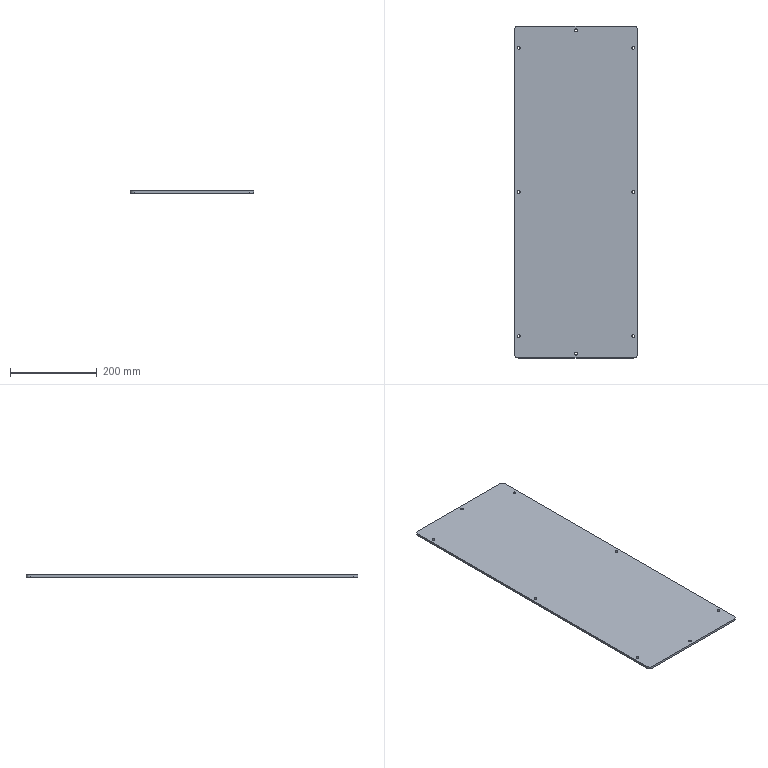Part | STEP file | 1 solid | 26 faces | box 284 x 764 x 5 mm | volume 1083123 mm3 | cylinder 20 | plane 6 | commonest cylinder face diameters 6.5 x16 20 x4